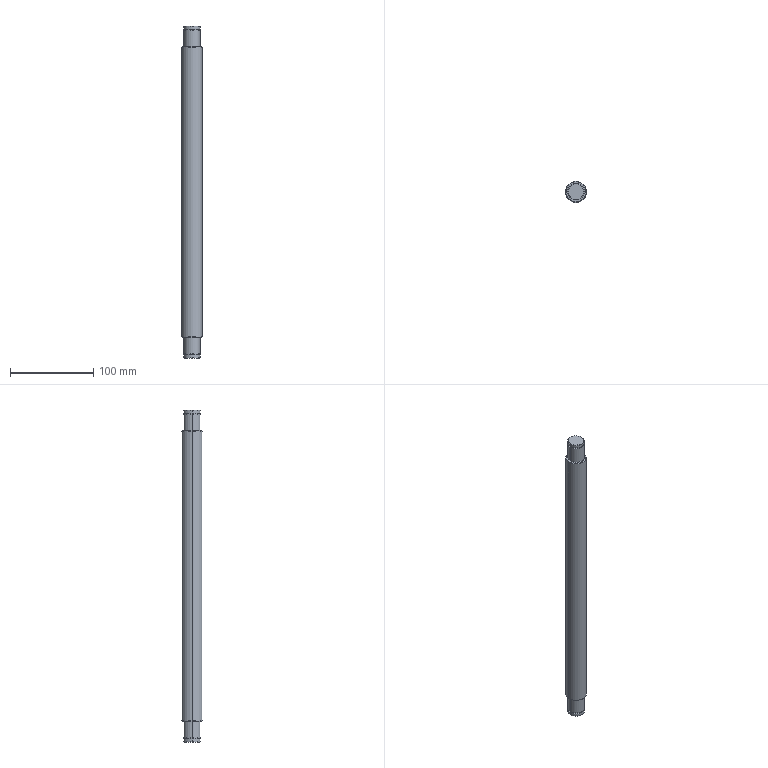Part | STEP file | X77-03305 | 1 solid | 30 faces | box 25 x 25 x 400 mm | volume 187252 mm3 | cylinder 14 | cone 8 | plane 8 | commonest cylinder face diameters 20 x8 17 x4 25 x2
STEP:
#1=CARTESIAN_POINT('',(10.,34775.535,-199.5));
#2=VERTEX_POINT('',#1);
#3=CARTESIAN_POINT('',(-10.,34775.535,-199.5));
#4=VERTEX_POINT('',#3);
#5=CARTESIAN_POINT('',(0.,34775.535,-199.5));
#6=DIRECTION('',(0.,0.,1.));
#7=DIRECTION('',(-1.,0.,0.));
#8=AXIS2_PLACEMENT_3D('',#5,#6,#7);
#9=CIRCLE('',#8,10.);
#10=EDGE_CURVE('',#2,#4,#9,.T.);
#11=ORIENTED_EDGE('',*,*,#10,.T.);
#12=CARTESIAN_POINT('',(-10.,34775.535,-196.3));
#13=VERTEX_POINT('',#12);
#14=CARTESIAN_POINT('',(-10.,34775.535,-200.));
#15=DIRECTION('',(0.,0.,1.));
#16=VECTOR('',#15,1000.);
#17=LINE('',#14,#16);
#18=EDGE_CURVE('',#4,#13,#17,.T.);
#19=ORIENTED_EDGE('',*,*,#18,.T.);
#20=CARTESIAN_POINT('',(10.,34775.535,-196.3));
#21=VERTEX_POINT('',#20);
#22=CARTESIAN_POINT('',(0.,34775.535,-196.3));
#23=DIRECTION('',(0.,0.,-1.));
#24=DIRECTION('',(-1.,0.,0.));
#25=AXIS2_PLACEMENT_3D('',#22,#23,#24);
#26=CIRCLE('',#25,10.);
#27=EDGE_CURVE('',#13,#21,#26,.T.);
#28=ORIENTED_EDGE('',*,*,#27,.T.);
#29=CARTESIAN_POINT('',(10.,34775.535,-200.));
#30=DIRECTION('',(0.,0.,1.));
#31=VECTOR('',#30,1000.);
#32=LINE('',#29,#31);
#33=EDGE_CURVE('',#2,#21,#32,.T.);
#34=ORIENTED_EDGE('',*,*,#33,.F.);
#35=EDGE_LOOP('',(#11,#19,#28,#34));
#36=FACE_OUTER_BOUND('',#35,.T.);
#37=CARTESIAN_POINT('',(0.,34775.535,-200.));
#38=DIRECTION('',(0.,0.,1.));
#39=DIRECTION('',(1.,0.,0.));
#40=AXIS2_PLACEMENT_3D('',#37,#38,#39);
#41=CYLINDRICAL_SURFACE('',#40,10.);
#42=ADVANCED_FACE('',(#36),#41,.T.);
#43=CARTESIAN_POINT('',(-9.5,34775.535,-200.));
#44=VERTEX_POINT('',#43);
#45=CARTESIAN_POINT('',(9.5,34775.535,-200.));
#46=VERTEX_POINT('',#45);
#47=CARTESIAN_POINT('',(0.,34775.535,-200.));
#48=DIRECTION('',(0.,0.,-1.));
#49=DIRECTION('',(-1.,0.,0.));
#50=AXIS2_PLACEMENT_3D('',#47,#48,#49);
#51=CIRCLE('',#50,9.5);
#52=EDGE_CURVE('',#44,#46,#51,.T.);
#53=ORIENTED_EDGE('',*,*,#52,.F.);
#54=CARTESIAN_POINT('',(-9.5,34775.535,-200.));
#55=DIRECTION('',(-0.7071,0.,0.7071));
#56=VECTOR('',#55,1000.);
#57=LINE('',#54,#56);
#58=EDGE_CURVE('',#44,#4,#57,.T.);
#59=ORIENTED_EDGE('',*,*,#58,.T.);
#60=ORIENTED_EDGE('',*,*,#10,.F.);
#61=CARTESIAN_POINT('',(9.5,34775.535,-200.));
#62=DIRECTION('',(0.7071,0.,0.7071));
#63=VECTOR('',#62,1000.);
#64=LINE('',#61,#63);
#65=EDGE_CURVE('',#46,#2,#64,.T.);
#66=ORIENTED_EDGE('',*,*,#65,.F.);
#67=EDGE_LOOP('',(#53,#59,#60,#66));
#68=FACE_OUTER_BOUND('',#67,.T.);
#69=CARTESIAN_POINT('',(0.,34775.535,-200.));
#70=DIRECTION('',(0.,0.,1.));
#71=DIRECTION('',(1.,0.,0.));
#72=AXIS2_PLACEMENT_3D('',#69,#70,#71);
#73=CONICAL_SURFACE('',#72,9.5,0.7854);
#74=ADVANCED_FACE('',(#68),#73,.T.);
#75=CARTESIAN_POINT('',(-8.5,34775.394,-195.));
#76=VERTEX_POINT('',#75);
#77=CARTESIAN_POINT('',(8.5,34775.394,-195.));
#78=VERTEX_POINT('',#77);
#79=CARTESIAN_POINT('',(0.,34775.394,-195.));
#80=DIRECTION('',(0.,0.,-1.));
#81=DIRECTION('',(-1.,0.,0.));
#82=AXIS2_PLACEMENT_3D('',#79,#80,#81);
#83=CIRCLE('',#82,8.5);
#84=EDGE_CURVE('',#76,#78,#83,.T.);
#85=ORIENTED_EDGE('',*,*,#84,.T.);
#86=CARTESIAN_POINT('',(8.5,34775.394,-196.3));
#87=VERTEX_POINT('',#86);
#88=CARTESIAN_POINT('',(8.5,34775.394,-207.249));
#89=DIRECTION('',(0.,0.,-1.));
#90=VECTOR('',#89,1000.);
#91=LINE('',#88,#90);
#92=EDGE_CURVE('',#78,#87,#91,.T.);
#93=ORIENTED_EDGE('',*,*,#92,.T.);
#94=CARTESIAN_POINT('',(-8.5,34775.394,-196.3));
#95=VERTEX_POINT('',#94);
#96=CARTESIAN_POINT('',(0.,34775.394,-196.3));
#97=DIRECTION('',(0.,0.,-1.));
#98=DIRECTION('',(-1.,0.,0.));
#99=AXIS2_PLACEMENT_3D('',#96,#97,#98);
#100=CIRCLE('',#99,8.5);
#101=EDGE_CURVE('',#95,#87,#100,.T.);
#102=ORIENTED_EDGE('',*,*,#101,.F.);
#103=CARTESIAN_POINT('',(-8.5,34775.394,-207.249));
#104=DIRECTION('',(0.,0.,-1.));
#105=VECTOR('',#104,1000.);
#106=LINE('',#103,#105);
#107=EDGE_CURVE('',#76,#95,#106,.T.);
#108=ORIENTED_EDGE('',*,*,#107,.F.);
#109=EDGE_LOOP('',(#85,#93,#102,#108));
#110=FACE_OUTER_BOUND('',#109,.T.);
#111=CARTESIAN_POINT('',(0.,34775.394,-207.249));
#112=DIRECTION('',(0.,0.,-1.));
#113=DIRECTION('',(-1.,0.,0.));
#114=AXIS2_PLACEMENT_3D('',#111,#112,#113);
#115=CYLINDRICAL_SURFACE('',#114,8.5);
#116=ADVANCED_FACE('',(#110),#115,.T.);
#117=CARTESIAN_POINT('',(-10.,34775.535,199.5));
#118=VERTEX_POINT('',#117);
#119=CARTESIAN_POINT('',(10.,34775.535,199.5));
#120=VERTEX_POINT('',#119);
#121=CARTESIAN_POINT('',(0.,34775.535,199.5));
#122=DIRECTION('',(0.,0.,-1.));
#123=DIRECTION('',(1.,0.,0.));
#124=AXIS2_PLACEMENT_3D('',#121,#122,#123);
#125=CIRCLE('',#124,10.);
#126=EDGE_CURVE('',#118,#120,#125,.T.);
#127=ORIENTED_EDGE('',*,*,#126,.T.);
#128=CARTESIAN_POINT('',(10.,34775.535,196.3));
#129=VERTEX_POINT('',#128);
#130=CARTESIAN_POINT('',(10.,34775.535,200.));
#131=DIRECTION('',(0.,0.,-1.));
#132=VECTOR('',#131,1000.);
#133=LINE('',#130,#132);
#134=EDGE_CURVE('',#120,#129,#133,.T.);
#135=ORIENTED_EDGE('',*,*,#134,.T.);
#136=CARTESIAN_POINT('',(-10.,34775.535,196.3));
#137=VERTEX_POINT('',#136);
#138=CARTESIAN_POINT('',(0.,34775.535,196.3));
#139=DIRECTION('',(0.,0.,1.));
#140=DIRECTION('',(1.,0.,0.));
#141=AXIS2_PLACEMENT_3D('',#138,#139,#140);
#142=CIRCLE('',#141,10.);
#143=EDGE_CURVE('',#129,#137,#142,.T.);
#144=ORIENTED_EDGE('',*,*,#143,.T.);
#145=CARTESIAN_POINT('',(-10.,34775.535,200.));
#146=DIRECTION('',(0.,0.,-1.));
#147=VECTOR('',#146,1000.);
#148=LINE('',#145,#147);
#149=EDGE_CURVE('',#118,#137,#148,.T.);
#150=ORIENTED_EDGE('',*,*,#149,.F.);
#151=EDGE_LOOP('',(#127,#135,#144,#150));
#152=FACE_OUTER_BOUND('',#151,.T.);
#153=CARTESIAN_POINT('',(0.,34775.535,200.));
#154=DIRECTION('',(0.,0.,-1.));
#155=DIRECTION('',(-1.,0.,0.));
#156=AXIS2_PLACEMENT_3D('',#153,#154,#155);
#157=CYLINDRICAL_SURFACE('',#156,10.);
#158=ADVANCED_FACE('',(#152),#157,.T.);
#159=CARTESIAN_POINT('',(9.5,34775.535,200.));
#160=VERTEX_POINT('',#159);
#161=CARTESIAN_POINT('',(-9.5,34775.535,200.));
#162=VERTEX_POINT('',#161);
#163=CARTESIAN_POINT('',(0.,34775.535,200.));
#164=DIRECTION('',(0.,0.,1.));
#165=DIRECTION('',(1.,0.,0.));
#166=AXIS2_PLACEMENT_3D('',#163,#164,#165);
#167=CIRCLE('',#166,9.5);
#168=EDGE_CURVE('',#160,#162,#167,.T.);
#169=ORIENTED_EDGE('',*,*,#168,.F.);
#170=CARTESIAN_POINT('',(9.5,34775.535,200.));
#171=DIRECTION('',(0.7071,0.,-0.7071));
#172=VECTOR('',#171,1000.);
#173=LINE('',#170,#172);
#174=EDGE_CURVE('',#160,#120,#173,.T.);
#175=ORIENTED_EDGE('',*,*,#174,.T.);
#176=ORIENTED_EDGE('',*,*,#126,.F.);
#177=CARTESIAN_POINT('',(-9.5,34775.535,200.));
#178=DIRECTION('',(-0.7071,0.,-0.7071));
#179=VECTOR('',#178,1000.);
#180=LINE('',#177,#179);
#181=EDGE_CURVE('',#162,#118,#180,.T.);
#182=ORIENTED_EDGE('',*,*,#181,.F.);
#183=EDGE_LOOP('',(#169,#175,#176,#182));
#184=FACE_OUTER_BOUND('',#183,.T.);
#185=CARTESIAN_POINT('',(0.,34775.535,200.));
#186=DIRECTION('',(0.,0.,-1.));
#187=DIRECTION('',(-1.,0.,0.));
#188=AXIS2_PLACEMENT_3D('',#185,#186,#187);
#189=CONICAL_SURFACE('',#188,9.5,0.7854);
#190=ADVANCED_FACE('',(#184),#189,.T.);
#191=CARTESIAN_POINT('',(-8.5,34775.394,196.3));
#192=VERTEX_POINT('',#191);
#193=CARTESIAN_POINT('',(8.5,34775.394,196.3));
#194=VERTEX_POINT('',#193);
#195=CARTESIAN_POINT('',(0.,34775.394,196.3));
#196=DIRECTION('',(0.,0.,-1.));
#197=DIRECTION('',(-1.,0.,0.));
#198=AXIS2_PLACEMENT_3D('',#195,#196,#197);
#199=CIRCLE('',#198,8.5);
#200=EDGE_CURVE('',#192,#194,#199,.T.);
#201=ORIENTED_EDGE('',*,*,#200,.T.);
#202=CARTESIAN_POINT('',(8.5,34775.394,195.));
#203=VERTEX_POINT('',#202);
#204=CARTESIAN_POINT('',(8.5,34775.394,-207.249));
#205=DIRECTION('',(0.,0.,-1.));
#206=VECTOR('',#205,1000.);
#207=LINE('',#204,#206);
#208=EDGE_CURVE('',#194,#203,#207,.T.);
#209=ORIENTED_EDGE('',*,*,#208,.T.);
#210=CARTESIAN_POINT('',(-8.5,34775.394,195.));
#211=VERTEX_POINT('',#210);
#212=CARTESIAN_POINT('',(0.,34775.394,195.));
#213=DIRECTION('',(0.,0.,-1.));
#214=DIRECTION('',(-1.,0.,0.));
#215=AXIS2_PLACEMENT_3D('',#212,#213,#214);
#216=CIRCLE('',#215,8.5);
#217=EDGE_CURVE('',#211,#203,#216,.T.);
#218=ORIENTED_EDGE('',*,*,#217,.F.);
#219=CARTESIAN_POINT('',(-8.5,34775.394,-207.249));
#220=DIRECTION('',(0.,0.,-1.));
#221=VECTOR('',#220,1000.);
#222=LINE('',#219,#221);
#223=EDGE_CURVE('',#192,#211,#222,.T.);
#224=ORIENTED_EDGE('',*,*,#223,.F.);
#225=EDGE_LOOP('',(#201,#209,#218,#224));
#226=FACE_OUTER_BOUND('',#225,.T.);
#227=CARTESIAN_POINT('',(0.,34775.394,-207.249));
#228=DIRECTION('',(0.,0.,-1.));
#229=DIRECTION('',(-1.,0.,0.));
#230=AXIS2_PLACEMENT_3D('',#227,#228,#229);
#231=CYLINDRICAL_SURFACE('',#230,8.5);
#232=ADVANCED_FACE('',(#226),#231,.T.);
#233=CARTESIAN_POINT('',(12.,34775.535,175.));
#234=VERTEX_POINT('',#233);
#235=CARTESIAN_POINT('',(-12.,34775.535,175.));
#236=VERTEX_POINT('',#235);
#237=CARTESIAN_POINT('',(0.,34775.535,175.));
#238=DIRECTION('',(0.,0.,1.));
#239=DIRECTION('',(1.,0.,0.));
#240=AXIS2_PLACEMENT_3D('',#237,#238,#239);
#241=CIRCLE('',#240,12.);
#242=EDGE_CURVE('',#234,#236,#241,.T.);
#243=ORIENTED_EDGE('',*,*,#242,.F.);
#244=CARTESIAN_POINT('',(12.5,34775.535,174.5));
#245=VERTEX_POINT('',#244);
#246=CARTESIAN_POINT('',(12.,34775.535,175.));
#247=DIRECTION('',(0.7071,0.,-0.7071));
#248=VECTOR('',#247,1000.);
#249=LINE('',#246,#248);
#250=EDGE_CURVE('',#234,#245,#249,.T.);
#251=ORIENTED_EDGE('',*,*,#250,.T.);
#252=CARTESIAN_POINT('',(-12.5,34775.535,174.5));
#253=VERTEX_POINT('',#252);
#254=CARTESIAN_POINT('',(0.,34775.535,174.5));
#255=DIRECTION('',(0.,0.,-1.));
#256=DIRECTION('',(1.,0.,0.));
#257=AXIS2_PLACEMENT_3D('',#254,#255,#256);
#258=CIRCLE('',#257,12.5);
#259=EDGE_CURVE('',#253,#245,#258,.T.);
#260=ORIENTED_EDGE('',*,*,#259,.F.);
#261=CARTESIAN_POINT('',(-12.,34775.535,175.));
#262=DIRECTION('',(-0.7071,0.,-0.7071));
#263=VECTOR('',#262,1000.);
#264=LINE('',#261,#263);
#265=EDGE_CURVE('',#236,#253,#264,.T.);
#266=ORIENTED_EDGE('',*,*,#265,.F.);
#267=EDGE_LOOP('',(#243,#251,#260,#266));
#268=FACE_OUTER_BOUND('',#267,.T.);
#269=CARTESIAN_POINT('',(0.,34775.535,175.));
#270=DIRECTION('',(0.,0.,-1.));
#271=DIRECTION('',(-1.,0.,0.));
#272=AXIS2_PLACEMENT_3D('',#269,#270,#271);
#273=CONICAL_SURFACE('',#272,12.,0.7854);
#274=ADVANCED_FACE('',(#268),#273,.T.);
#275=CARTESIAN_POINT('',(-12.,34775.535,-175.));
#276=VERTEX_POINT('',#275);
#277=CARTESIAN_POINT('',(12.,34775.535,-175.));
#278=VERTEX_POINT('',#277);
#279=CARTESIAN_POINT('',(0.,34775.535,-175.));
#280=DIRECTION('',(0.,0.,-1.));
#281=DIRECTION('',(1.,0.,0.));
#282=AXIS2_PLACEMENT_3D('',#279,#280,#281);
#283=CIRCLE('',#282,12.);
#284=EDGE_CURVE('',#276,#278,#283,.T.);
#285=ORIENTED_EDGE('',*,*,#284,.F.);
#286=CARTESIAN_POINT('',(-12.5,34775.535,-174.5));
#287=VERTEX_POINT('',#286);
#288=CARTESIAN_POINT('',(-12.5,34775.535,-174.5));
#289=DIRECTION('',(-0.7071,0.,0.7071));
#290=VECTOR('',#289,1000.);
#291=LINE('',#288,#290);
#292=EDGE_CURVE('',#276,#287,#291,.T.);
#293=ORIENTED_EDGE('',*,*,#292,.T.);
#294=CARTESIAN_POINT('',(12.5,34775.535,-174.5));
#295=VERTEX_POINT('',#294);
#296=CARTESIAN_POINT('',(0.,34775.535,-174.5));
#297=DIRECTION('',(0.,0.,1.));
#298=DIRECTION('',(1.,0.,0.));
#299=AXIS2_PLACEMENT_3D('',#296,#297,#298);
#300=CIRCLE('',#299,12.5);
#301=EDGE_CURVE('',#295,#287,#300,.T.);
#302=ORIENTED_EDGE('',*,*,#301,.F.);
#303=CARTESIAN_POINT('',(12.5,34775.535,-174.5));
#304=DIRECTION('',(0.7071,0.,0.7071));
#305=VECTOR('',#304,1000.);
#306=LINE('',#303,#305);
#307=EDGE_CURVE('',#278,#295,#306,.T.);
#308=ORIENTED_EDGE('',*,*,#307,.F.);
#309=EDGE_LOOP('',(#285,#293,#302,#308));
#310=FACE_OUTER_BOUND('',#309,.T.);
#311=CARTESIAN_POINT('',(0.,34775.535,-174.5));
#312=DIRECTION('',(0.,0.,1.));
#313=DIRECTION('',(1.,0.,0.));
#314=AXIS2_PLACEMENT_3D('',#311,#312,#313);
#315=CONICAL_SURFACE('',#314,12.5,0.7854);
#316=ADVANCED_FACE('',(#310),#315,.T.);
#317=CARTESIAN_POINT('',(10.,34775.535,-195.));
#318=VERTEX_POINT('',#317);
#319=CARTESIAN_POINT('',(-10.,34775.535,-195.));
#320=VERTEX_POINT('',#319);
#321=CARTESIAN_POINT('',(0.,34775.535,-195.));
#322=DIRECTION('',(0.,0.,1.));
#323=DIRECTION('',(1.,0.,0.));
#324=AXIS2_PLACEMENT_3D('',#321,#322,#323);
#325=CIRCLE('',#324,10.);
#326=EDGE_CURVE('',#318,#320,#325,.T.);
#327=ORIENTED_EDGE('',*,*,#326,.T.);
#328=CARTESIAN_POINT('',(-10.,34775.535,-175.));
#329=VERTEX_POINT('',#328);
#330=CARTESIAN_POINT('',(-10.,34775.535,-200.));
#331=DIRECTION('',(0.,0.,1.));
#332=VECTOR('',#331,1000.);
#333=LINE('',#330,#332);
#334=EDGE_CURVE('',#320,#329,#333,.T.);
#335=ORIENTED_EDGE('',*,*,#334,.T.);
#336=CARTESIAN_POINT('',(10.,34775.535,-175.));
#337=VERTEX_POINT('',#336);
#338=CARTESIAN_POINT('',(0.,34775.535,-175.));
#339=DIRECTION('',(0.,0.,-1.));
#340=DIRECTION('',(1.,0.,0.));
#341=AXIS2_PLACEMENT_3D('',#338,#339,#340);
#342=CIRCLE('',#341,10.);
#343=EDGE_CURVE('',#329,#337,#342,.T.);
#344=ORIENTED_EDGE('',*,*,#343,.T.);
#345=CARTESIAN_POINT('',(10.,34775.535,-200.));
#346=DIRECTION('',(0.,0.,1.));
#347=VECTOR('',#346,1000.);
#348=LINE('',#345,#347);
#349=EDGE_CURVE('',#318,#337,#348,.T.);
#350=ORIENTED_EDGE('',*,*,#349,.F.);
#351=EDGE_LOOP('',(#327,#335,#344,#350));
#352=FACE_OUTER_BOUND('',#351,.T.);
#353=CARTESIAN_POINT('',(0.,34775.535,-200.));
#354=DIRECTION('',(0.,0.,1.));
#355=DIRECTION('',(1.,0.,0.));
#356=AXIS2_PLACEMENT_3D('',#353,#354,#355);
#357=CYLINDRICAL_SURFACE('',#356,10.);
#358=ADVANCED_FACE('',(#352),#357,.T.);
#359=CARTESIAN_POINT('',(-10.,34775.535,195.));
#360=VERTEX_POINT('',#359);
#361=CARTESIAN_POINT('',(10.,34775.535,195.));
#362=VERTEX_POINT('',#361);
#363=CARTESIAN_POINT('',(0.,34775.535,195.));
#364=DIRECTION('',(0.,0.,-1.));
#365=DIRECTION('',(-1.,0.,0.));
#366=AXIS2_PLACEMENT_3D('',#363,#364,#365);
#367=CIRCLE('',#366,10.);
#368=EDGE_CURVE('',#360,#362,#367,.T.);
#369=ORIENTED_EDGE('',*,*,#368,.T.);
#370=CARTESIAN_POINT('',(10.,34775.535,175.));
#371=VERTEX_POINT('',#370);
#372=CARTESIAN_POINT('',(10.,34775.535,200.));
#373=DIRECTION('',(0.,0.,-1.));
#374=VECTOR('',#373,1000.);
#375=LINE('',#372,#374);
#376=EDGE_CURVE('',#362,#371,#375,.T.);
#377=ORIENTED_EDGE('',*,*,#376,.T.);
#378=CARTESIAN_POINT('',(-10.,34775.535,175.));
#379=VERTEX_POINT('',#378);
#380=CARTESIAN_POINT('',(0.,34775.535,175.));
#381=DIRECTION('',(0.,0.,1.));
#382=DIRECTION('',(1.,0.,0.));
#383=AXIS2_PLACEMENT_3D('',#380,#381,#382);
#384=CIRCLE('',#383,10.);
#385=EDGE_CURVE('',#371,#379,#384,.T.);
#386=ORIENTED_EDGE('',*,*,#385,.T.);
#387=CARTESIAN_POINT('',(-10.,34775.535,200.));
#388=DIRECTION('',(0.,0.,-1.));
#389=VECTOR('',#388,1000.);
#390=LINE('',#387,#389);
#391=EDGE_CURVE('',#360,#379,#390,.T.);
#392=ORIENTED_EDGE('',*,*,#391,.F.);
#393=EDGE_LOOP('',(#369,#377,#386,#392));
#394=FACE_OUTER_BOUND('',#393,.T.);
#395=CARTESIAN_POINT('',(0.,34775.535,200.));
#396=DIRECTION('',(0.,0.,-1.));
#397=DIRECTION('',(-1.,0.,0.));
#398=AXIS2_PLACEMENT_3D('',#395,#396,#397);
#399=CYLINDRICAL_SURFACE('',#398,10.);
#400=ADVANCED_FACE('',(#394),#399,.T.);
#401=ORIENTED_EDGE('',*,*,#301,.T.);
#402=CARTESIAN_POINT('',(-12.5,34775.535,-175.));
#403=DIRECTION('',(0.,0.,1.));
#404=VECTOR('',#403,1000.);
#405=LINE('',#402,#404);
#406=EDGE_CURVE('',#287,#253,#405,.T.);
#407=ORIENTED_EDGE('',*,*,#406,.T.);
#408=ORIENTED_EDGE('',*,*,#259,.T.);
#409=CARTESIAN_POINT('',(12.5,34775.535,-175.));
#410=DIRECTION('',(0.,0.,1.));
#411=VECTOR('',#410,1000.);
#412=LINE('',#409,#411);
#413=EDGE_CURVE('',#295,#245,#412,.T.);
#414=ORIENTED_EDGE('',*,*,#413,.F.);
#415=EDGE_LOOP('',(#401,#407,#408,#414));
#416=FACE_OUTER_BOUND('',#415,.T.);
#417=CARTESIAN_POINT('',(0.,34775.535,-175.));
#418=DIRECTION('',(0.,0.,1.));
#419=DIRECTION('',(1.,0.,0.));
#420=AXIS2_PLACEMENT_3D('',#417,#418,#419);
#421=CYLINDRICAL_SURFACE('',#420,12.5);
#422=ADVANCED_FACE('',(#416),#421,.T.);
#423=CARTESIAN_POINT('',(0.,34775.535,-175.));
#424=DIRECTION('',(0.,0.,-1.));
#425=DIRECTION('',(1.,0.,0.));
#426=AXIS2_PLACEMENT_3D('',#423,#424,#425);
#427=CIRCLE('',#426,12.);
#428=EDGE_CURVE('',#278,#276,#427,.T.);
#429=ORIENTED_EDGE('',*,*,#428,.T.);
#430=ORIENTED_EDGE('',*,*,#284,.T.);
#431=EDGE_LOOP('',(#429,#430));
#432=FACE_OUTER_BOUND('',#431,.T.);
#433=CARTESIAN_POINT('',(0.,34775.535,-175.));
#434=DIRECTION('',(0.,0.,-1.));
#435=DIRECTION('',(1.,0.,0.));
#436=AXIS2_PLACEMENT_3D('',#433,#434,#435);
#437=CIRCLE('',#436,10.);
#438=EDGE_CURVE('',#337,#329,#437,.T.);
#439=ORIENTED_EDGE('',*,*,#438,.F.);
#440=ORIENTED_EDGE('',*,*,#343,.F.);
#441=EDGE_LOOP('',(#439,#440));
#442=FACE_BOUND('',#441,.T.);
#443=CARTESIAN_POINT('',(0.,34775.535,-175.));
#444=DIRECTION('',(0.,0.,1.));
#445=DIRECTION('',(1.,0.,0.));
#446=AXIS2_PLACEMENT_3D('',#443,#444,#445);
#447=PLANE('',#446);
#448=ADVANCED_FACE('',(#432,#442),#447,.F.);
#449=CARTESIAN_POINT('',(0.,34775.535,175.));
#450=DIRECTION('',(0.,0.,1.));
#451=DIRECTION('',(1.,0.,0.));
#452=AXIS2_PLACEMENT_3D('',#449,#450,#451);
#453=CIRCLE('',#452,12.);
#454=EDGE_CURVE('',#236,#234,#453,.T.);
#455=ORIENTED_EDGE('',*,*,#454,.T.);
#456=ORIENTED_EDGE('',*,*,#242,.T.);
#457=EDGE_LOOP('',(#455,#456));
#458=FACE_OUTER_BOUND('',#457,.T.);
#459=CARTESIAN_POINT('',(0.,34775.535,175.));
#460=DIRECTION('',(0.,0.,1.));
#461=DIRECTION('',(1.,0.,0.));
#462=AXIS2_PLACEMENT_3D('',#459,#460,#461);
#463=CIRCLE('',#462,10.);
#464=EDGE_CURVE('',#379,#371,#463,.T.);
#465=ORIENTED_EDGE('',*,*,#464,.F.);
#466=ORIENTED_EDGE('',*,*,#385,.F.);
#467=EDGE_LOOP('',(#465,#466));
#468=FACE_BOUND('',#467,.T.);
#469=CARTESIAN_POINT('',(0.,34775.535,175.));
#470=DIRECTION('',(0.,0.,1.));
#471=DIRECTION('',(1.,0.,0.));
#472=AXIS2_PLACEMENT_3D('',#469,#470,#471);
#473=PLANE('',#472);
#474=ADVANCED_FACE('',(#458,#468),#473,.T.);
#475=ORIENTED_EDGE('',*,*,#406,.F.);
#476=CARTESIAN_POINT('',(0.,34775.535,-174.5));
#477=DIRECTION('',(0.,0.,1.));
#478=DIRECTION('',(1.,0.,0.));
#479=AXIS2_PLACEMENT_3D('',#476,#477,#478);
#480=CIRCLE('',#479,12.5);
#481=EDGE_CURVE('',#287,#295,#480,.T.);
#482=ORIENTED_EDGE('',*,*,#481,.T.);
#483=ORIENTED_EDGE('',*,*,#413,.T.);
#484=CARTESIAN_POINT('',(0.,34775.535,174.5));
#485=DIRECTION('',(0.,0.,-1.));
#486=DIRECTION('',(1.,0.,0.));
#487=AXIS2_PLACEMENT_3D('',#484,#485,#486);
#488=CIRCLE('',#487,12.5);
#489=EDGE_CURVE('',#245,#253,#488,.T.);
#490=ORIENTED_EDGE('',*,*,#489,.T.);
#491=EDGE_LOOP('',(#475,#482,#483,#490));
#492=FACE_OUTER_BOUND('',#491,.T.);
#493=CARTESIAN_POINT('',(0.,34775.535,-175.));
#494=DIRECTION('',(0.,0.,1.));
#495=DIRECTION('',(1.,0.,0.));
#496=AXIS2_PLACEMENT_3D('',#493,#494,#495);
#497=CYLINDRICAL_SURFACE('',#496,12.5);
#498=ADVANCED_FACE('',(#492),#497,.T.);
#499=ORIENTED_EDGE('',*,*,#376,.F.);
#500=CARTESIAN_POINT('',(0.,34775.535,195.));
#501=DIRECTION('',(0.,0.,-1.));
#502=DIRECTION('',(-1.,0.,0.));
#503=AXIS2_PLACEMENT_3D('',#500,#501,#502);
#504=CIRCLE('',#503,10.);
#505=EDGE_CURVE('',#362,#360,#504,.T.);
#506=ORIENTED_EDGE('',*,*,#505,.T.);
#507=ORIENTED_EDGE('',*,*,#391,.T.);
#508=ORIENTED_EDGE('',*,*,#464,.T.);
#509=EDGE_LOOP('',(#499,#506,#507,#508));
#510=FACE_OUTER_BOUND('',#509,.T.);
#511=CARTESIAN_POINT('',(0.,34775.535,200.));
#512=DIRECTION('',(0.,0.,-1.));
#513=DIRECTION('',(-1.,0.,0.));
#514=AXIS2_PLACEMENT_3D('',#511,#512,#513);
#515=CYLINDRICAL_SURFACE('',#514,10.);
#516=ADVANCED_FACE('',(#510),#515,.T.);
#517=ORIENTED_EDGE('',*,*,#334,.F.);
#518=CARTESIAN_POINT('',(0.,34775.535,-195.));
#519=DIRECTION('',(0.,0.,1.));
#520=DIRECTION('',(1.,0.,0.));
#521=AXIS2_PLACEMENT_3D('',#518,#519,#520);
#522=CIRCLE('',#521,10.);
#523=EDGE_CURVE('',#320,#318,#522,.T.);
#524=ORIENTED_EDGE('',*,*,#523,.T.);
#525=ORIENTED_EDGE('',*,*,#349,.T.);
#526=ORIENTED_EDGE('',*,*,#438,.T.);
#527=EDGE_LOOP('',(#517,#524,#525,#526));
#528=FACE_OUTER_BOUND('',#527,.T.);
#529=CARTESIAN_POINT('',(0.,34775.535,-200.));
#530=DIRECTION('',(0.,0.,1.));
#531=DIRECTION('',(1.,0.,0.));
#532=AXIS2_PLACEMENT_3D('',#529,#530,#531);
#533=CYLINDRICAL_SURFACE('',#532,10.);
#534=ADVANCED_FACE('',(#528),#533,.T.);
#535=ORIENTED_EDGE('',*,*,#292,.F.);
#536=ORIENTED_EDGE('',*,*,#428,.F.);
#537=ORIENTED_EDGE('',*,*,#307,.T.);
#538=ORIENTED_EDGE('',*,*,#481,.F.);
#539=EDGE_LOOP('',(#535,#536,#537,#538));
#540=FACE_OUTER_BOUND('',#539,.T.);
#541=CARTESIAN_POINT('',(0.,34775.535,-174.5));
#542=DIRECTION('',(0.,0.,1.));
#543=DIRECTION('',(1.,0.,0.));
#544=AXIS2_PLACEMENT_3D('',#541,#542,#543);
#545=CONICAL_SURFACE('',#544,12.5,0.7854);
#546=ADVANCED_FACE('',(#540),#545,.T.);
#547=ORIENTED_EDGE('',*,*,#250,.F.);
#548=ORIENTED_EDGE('',*,*,#454,.F.);
#549=ORIENTED_EDGE('',*,*,#265,.T.);
#550=ORIENTED_EDGE('',*,*,#489,.F.);
#551=EDGE_LOOP('',(#547,#548,#549,#550));
#552=FACE_OUTER_BOUND('',#551,.T.);
#553=CARTESIAN_POINT('',(0.,34775.535,175.));
#554=DIRECTION('',(0.,0.,-1.));
#555=DIRECTION('',(-1.,0.,0.));
#556=AXIS2_PLACEMENT_3D('',#553,#554,#555);
#557=CONICAL_SURFACE('',#556,12.,0.7854);
#558=ADVANCED_FACE('',(#552),#557,.T.);
#559=ORIENTED_EDGE('',*,*,#200,.F.);
#560=CARTESIAN_POINT('',(0.,34775.394,196.3));
#561=DIRECTION('',(0.,0.,-1.));
#562=DIRECTION('',(-1.,0.,0.));
#563=AXIS2_PLACEMENT_3D('',#560,#561,#562);
#564=CIRCLE('',#563,8.5);
#565=EDGE_CURVE('',#194,#192,#564,.T.);
#566=ORIENTED_EDGE('',*,*,#565,.F.);
#567=EDGE_LOOP('',(#559,#566));
#568=FACE_BOUND('',#567,.T.);
#569=CARTESIAN_POINT('',(0.,34775.535,196.3));
#570=DIRECTION('',(0.,0.,1.));
#571=DIRECTION('',(1.,0.,0.));
#572=AXIS2_PLACEMENT_3D('',#569,#570,#571);
#573=CIRCLE('',#572,10.);
#574=EDGE_CURVE('',#137,#129,#573,.T.);
#575=ORIENTED_EDGE('',*,*,#574,.F.);
#576=ORIENTED_EDGE('',*,*,#143,.F.);
#577=EDGE_LOOP('',(#575,#576));
#578=FACE_OUTER_BOUND('',#577,.T.);
#579=CARTESIAN_POINT('',(0.,34785.535,196.3));
#580=DIRECTION('',(0.,0.,1.));
#581=DIRECTION('',(1.,0.,0.));
#582=AXIS2_PLACEMENT_3D('',#579,#580,#581);
#583=PLANE('',#582);
#584=ADVANCED_FACE('',(#568,#578),#583,.F.);
#585=ORIENTED_EDGE('',*,*,#217,.T.);
#586=CARTESIAN_POINT('',(0.,34775.394,195.));
#587=DIRECTION('',(0.,0.,-1.));
#588=DIRECTION('',(-1.,0.,0.));
#589=AXIS2_PLACEMENT_3D('',#586,#587,#588);
#590=CIRCLE('',#589,8.5);
#591=EDGE_CURVE('',#203,#211,#590,.T.);
#592=ORIENTED_EDGE('',*,*,#591,.T.);
#593=EDGE_LOOP('',(#585,#592));
#594=FACE_BOUND('',#593,.T.);
#595=ORIENTED_EDGE('',*,*,#368,.F.);
#596=ORIENTED_EDGE('',*,*,#505,.F.);
#597=EDGE_LOOP('',(#595,#596));
#598=FACE_OUTER_BOUND('',#597,.T.);
#599=CARTESIAN_POINT('',(0.,34785.535,195.));
#600=DIRECTION('',(0.,0.,-1.));
#601=DIRECTION('',(-1.,0.,0.));
#602=AXIS2_PLACEMENT_3D('',#599,#600,#601);
#603=PLANE('',#602);
#604=ADVANCED_FACE('',(#594,#598),#603,.F.);
#605=ORIENTED_EDGE('',*,*,#208,.F.);
#606=ORIENTED_EDGE('',*,*,#565,.T.);
#607=ORIENTED_EDGE('',*,*,#223,.T.);
#608=ORIENTED_EDGE('',*,*,#591,.F.);
#609=EDGE_LOOP('',(#605,#606,#607,#608));
#610=FACE_OUTER_BOUND('',#609,.T.);
#611=CARTESIAN_POINT('',(0.,34775.394,-207.249));
#612=DIRECTION('',(0.,0.,-1.));
#613=DIRECTION('',(-1.,0.,0.));
#614=AXIS2_PLACEMENT_3D('',#611,#612,#613);
#615=CYLINDRICAL_SURFACE('',#614,8.5);
#616=ADVANCED_FACE('',(#610),#615,.T.);
#617=CARTESIAN_POINT('',(0.,34775.535,200.));
#618=DIRECTION('',(0.,0.,1.));
#619=DIRECTION('',(1.,0.,0.));
#620=AXIS2_PLACEMENT_3D('',#617,#618,#619);
#621=CIRCLE('',#620,9.5);
#622=EDGE_CURVE('',#162,#160,#621,.T.);
#623=ORIENTED_EDGE('',*,*,#622,.T.);
#624=ORIENTED_EDGE('',*,*,#168,.T.);
#625=EDGE_LOOP('',(#623,#624));
#626=FACE_OUTER_BOUND('',#625,.T.);
#627=CARTESIAN_POINT('',(0.,34775.535,200.));
#628=DIRECTION('',(0.,0.,1.));
#629=DIRECTION('',(1.,0.,0.));
#630=AXIS2_PLACEMENT_3D('',#627,#628,#629);
#631=PLANE('',#630);
#632=ADVANCED_FACE('',(#626),#631,.T.);
#633=ORIENTED_EDGE('',*,*,#174,.F.);
#634=ORIENTED_EDGE('',*,*,#622,.F.);
#635=ORIENTED_EDGE('',*,*,#181,.T.);
#636=CARTESIAN_POINT('',(0.,34775.535,199.5));
#637=DIRECTION('',(0.,0.,-1.));
#638=DIRECTION('',(1.,0.,0.));
#639=AXIS2_PLACEMENT_3D('',#636,#637,#638);
#640=CIRCLE('',#639,10.);
#641=EDGE_CURVE('',#120,#118,#640,.T.);
#642=ORIENTED_EDGE('',*,*,#641,.F.);
#643=EDGE_LOOP('',(#633,#634,#635,#642));
#644=FACE_OUTER_BOUND('',#643,.T.);
#645=CARTESIAN_POINT('',(0.,34775.535,200.));
#646=DIRECTION('',(0.,0.,-1.));
#647=DIRECTION('',(-1.,0.,0.));
#648=AXIS2_PLACEMENT_3D('',#645,#646,#647);
#649=CONICAL_SURFACE('',#648,9.5,0.7854);
#650=ADVANCED_FACE('',(#644),#649,.T.);
#651=ORIENTED_EDGE('',*,*,#134,.F.);
#652=ORIENTED_EDGE('',*,*,#641,.T.);
#653=ORIENTED_EDGE('',*,*,#149,.T.);
#654=ORIENTED_EDGE('',*,*,#574,.T.);
#655=EDGE_LOOP('',(#651,#652,#653,#654));
#656=FACE_OUTER_BOUND('',#655,.T.);
#657=CARTESIAN_POINT('',(0.,34775.535,200.));
#658=DIRECTION('',(0.,0.,-1.));
#659=DIRECTION('',(-1.,0.,0.));
#660=AXIS2_PLACEMENT_3D('',#657,#658,#659);
#661=CYLINDRICAL_SURFACE('',#660,10.);
#662=ADVANCED_FACE('',(#656),#661,.T.);
#663=ORIENTED_EDGE('',*,*,#101,.T.);
#664=CARTESIAN_POINT('',(0.,34775.394,-196.3));
#665=DIRECTION('',(0.,0.,-1.));
#666=DIRECTION('',(-1.,0.,0.));
#667=AXIS2_PLACEMENT_3D('',#664,#665,#666);
#668=CIRCLE('',#667,8.5);
#669=EDGE_CURVE('',#87,#95,#668,.T.);
#670=ORIENTED_EDGE('',*,*,#669,.T.);
#671=EDGE_LOOP('',(#663,#670));
#672=FACE_BOUND('',#671,.T.);
#673=CARTESIAN_POINT('',(0.,34775.535,-196.3));
#674=DIRECTION('',(0.,0.,-1.));
#675=DIRECTION('',(-1.,0.,0.));
#676=AXIS2_PLACEMENT_3D('',#673,#674,#675);
#677=CIRCLE('',#676,10.);
#678=EDGE_CURVE('',#21,#13,#677,.T.);
#679=ORIENTED_EDGE('',*,*,#678,.F.);
#680=ORIENTED_EDGE('',*,*,#27,.F.);
#681=EDGE_LOOP('',(#679,#680));
#682=FACE_OUTER_BOUND('',#681,.T.);
#683=CARTESIAN_POINT('',(0.,34785.535,-196.3));
#684=DIRECTION('',(0.,0.,-1.));
#685=DIRECTION('',(-1.,0.,0.));
#686=AXIS2_PLACEMENT_3D('',#683,#684,#685);
#687=PLANE('',#686);
#688=ADVANCED_FACE('',(#672,#682),#687,.F.);
#689=ORIENTED_EDGE('',*,*,#84,.F.);
#690=CARTESIAN_POINT('',(0.,34775.394,-195.));
#691=DIRECTION('',(0.,0.,-1.));
#692=DIRECTION('',(-1.,0.,0.));
#693=AXIS2_PLACEMENT_3D('',#690,#691,#692);
#694=CIRCLE('',#693,8.5);
#695=EDGE_CURVE('',#78,#76,#694,.T.);
#696=ORIENTED_EDGE('',*,*,#695,.F.);
#697=EDGE_LOOP('',(#689,#696));
#698=FACE_BOUND('',#697,.T.);
#699=ORIENTED_EDGE('',*,*,#326,.F.);
#700=ORIENTED_EDGE('',*,*,#523,.F.);
#701=EDGE_LOOP('',(#699,#700));
#702=FACE_OUTER_BOUND('',#701,.T.);
#703=CARTESIAN_POINT('',(0.,34785.535,-195.));
#704=DIRECTION('',(0.,0.,1.));
#705=DIRECTION('',(1.,0.,0.));
#706=AXIS2_PLACEMENT_3D('',#703,#704,#705);
#707=PLANE('',#706);
#708=ADVANCED_FACE('',(#698,#702),#707,.F.);
#709=ORIENTED_EDGE('',*,*,#92,.F.);
#710=ORIENTED_EDGE('',*,*,#695,.T.);
#711=ORIENTED_EDGE('',*,*,#107,.T.);
#712=ORIENTED_EDGE('',*,*,#669,.F.);
#713=EDGE_LOOP('',(#709,#710,#711,#712));
#714=FACE_OUTER_BOUND('',#713,.T.);
#715=CARTESIAN_POINT('',(0.,34775.394,-207.249));
#716=DIRECTION('',(0.,0.,-1.));
#717=DIRECTION('',(-1.,0.,0.));
#718=AXIS2_PLACEMENT_3D('',#715,#716,#717);
#719=CYLINDRICAL_SURFACE('',#718,8.5);
#720=ADVANCED_FACE('',(#714),#719,.T.);
#721=CARTESIAN_POINT('',(0.,34775.535,-200.));
#722=DIRECTION('',(0.,0.,-1.));
#723=DIRECTION('',(-1.,0.,0.));
#724=AXIS2_PLACEMENT_3D('',#721,#722,#723);
#725=CIRCLE('',#724,9.5);
#726=EDGE_CURVE('',#46,#44,#725,.T.);
#727=ORIENTED_EDGE('',*,*,#726,.T.);
#728=ORIENTED_EDGE('',*,*,#52,.T.);
#729=EDGE_LOOP('',(#727,#728));
#730=FACE_OUTER_BOUND('',#729,.T.);
#731=CARTESIAN_POINT('',(0.,34775.535,-200.));
#732=DIRECTION('',(0.,0.,-1.));
#733=DIRECTION('',(-1.,0.,0.));
#734=AXIS2_PLACEMENT_3D('',#731,#732,#733);
#735=PLANE('',#734);
#736=ADVANCED_FACE('',(#730),#735,.T.);
#737=ORIENTED_EDGE('',*,*,#58,.F.);
#738=ORIENTED_EDGE('',*,*,#726,.F.);
#739=ORIENTED_EDGE('',*,*,#65,.T.);
#740=CARTESIAN_POINT('',(0.,34775.535,-199.5));
#741=DIRECTION('',(0.,0.,1.));
#742=DIRECTION('',(-1.,0.,0.));
#743=AXIS2_PLACEMENT_3D('',#740,#741,#742);
#744=CIRCLE('',#743,10.);
#745=EDGE_CURVE('',#4,#2,#744,.T.);
#746=ORIENTED_EDGE('',*,*,#745,.F.);
#747=EDGE_LOOP('',(#737,#738,#739,#746));
#748=FACE_OUTER_BOUND('',#747,.T.);
#749=CARTESIAN_POINT('',(0.,34775.535,-200.));
#750=DIRECTION('',(0.,0.,1.));
#751=DIRECTION('',(1.,0.,0.));
#752=AXIS2_PLACEMENT_3D('',#749,#750,#751);
#753=CONICAL_SURFACE('',#752,9.5,0.7854);
#754=ADVANCED_FACE('',(#748),#753,.T.);
#755=ORIENTED_EDGE('',*,*,#18,.F.);
#756=ORIENTED_EDGE('',*,*,#745,.T.);
#757=ORIENTED_EDGE('',*,*,#33,.T.);
#758=ORIENTED_EDGE('',*,*,#678,.T.);
#759=EDGE_LOOP('',(#755,#756,#757,#758));
#760=FACE_OUTER_BOUND('',#759,.T.);
#761=CARTESIAN_POINT('',(0.,34775.535,-200.));
#762=DIRECTION('',(0.,0.,1.));
#763=DIRECTION('',(1.,0.,0.));
#764=AXIS2_PLACEMENT_3D('',#761,#762,#763);
#765=CYLINDRICAL_SURFACE('',#764,10.);
#766=ADVANCED_FACE('',(#760),#765,.T.);
#767=CLOSED_SHELL('',(#42,#74,#116,#158,#190,#232,#274,#316,#358,#400,#422,#448,#474,#498,#516,#534,#546,#558,#584,#604,#616,#632,#650,#662,#688,#708,#720,#736,#754,#766));
#768=MANIFOLD_SOLID_BREP('',#767);
#769=CARTESIAN_POINT('',(0.,0.,0.));
#770=DIRECTION('',(0.,0.,1.));
#771=DIRECTION('',(1.,0.,0.));
#772=AXIS2_PLACEMENT_3D('',#769,#770,#771);
#773=(LENGTH_UNIT()NAMED_UNIT(*)SI_UNIT(.MILLI.,.METRE.));
#774=UNCERTAINTY_MEASURE_WITH_UNIT(LENGTH_MEASURE(0.00001),#773,'','');
#775=(NAMED_UNIT(*)PLANE_ANGLE_UNIT()SI_UNIT($,.RADIAN.));
#776=(NAMED_UNIT(*)SI_UNIT($,.STERADIAN.)SOLID_ANGLE_UNIT());
#777=(GEOMETRIC_REPRESENTATION_CONTEXT(3)GLOBAL_UNCERTAINTY_ASSIGNED_CONTEXT((#774))GLOBAL_UNIT_ASSIGNED_CONTEXT((#773,#775,#776))REPRESENTATION_CONTEXT('',''));
#778=ADVANCED_BREP_SHAPE_REPRESENTATION('',(#768,#772),#777);